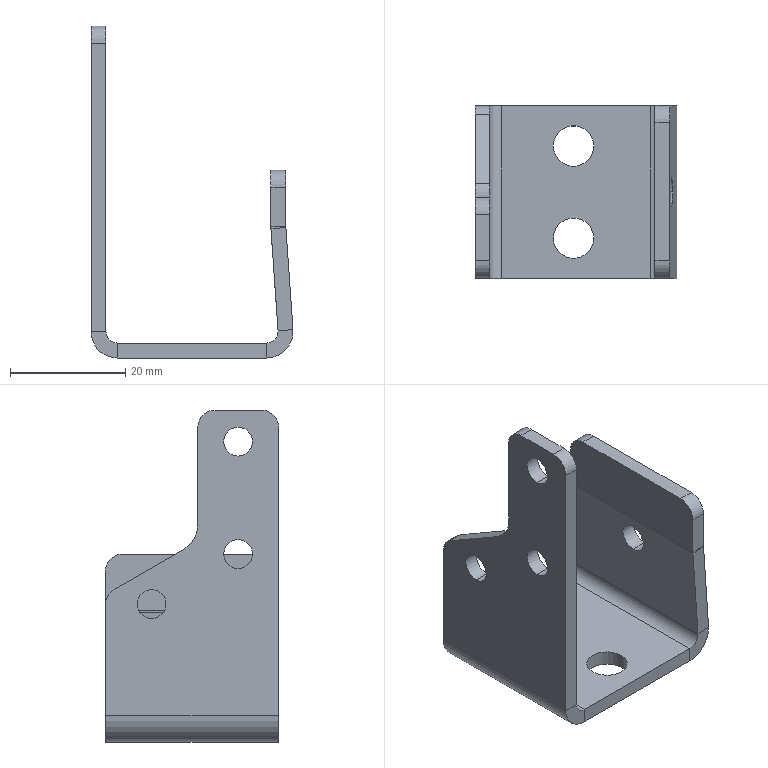Part | STEP file | SOPORTE RESORTE 1 | 1 solid | 50 faces | box 35.055 x 30 x 57.6 mm | volume 7586 mm3 | plane 26 | cylinder 24 | commonest cylinder face diameters 5 x8 6 x5 7 x4 4 x3 9.2 x3 10 x1
STEP:
#1=CARTESIAN_POINT('',(14.241,15.,3.502));
#2=VERTEX_POINT('',#1);
#3=CARTESIAN_POINT('',(14.59,15.,-1.486));
#4=VERTEX_POINT('',#3);
#5=CARTESIAN_POINT('',(14.416,15.,1.008));
#6=DIRECTION('',(0.9976,0.,0.06976));
#7=DIRECTION('',(0.06976,0.,-0.9976));
#8=AXIS2_PLACEMENT_3D('',#5,#6,#7);
#9=CIRCLE('',#8,2.5);
#10=EDGE_CURVE('',#2,#4,#9,.T.);
#11=ORIENTED_EDGE('',*,*,#10,.F.);
#12=CARTESIAN_POINT('',(16.835,15.,3.683));
#13=VERTEX_POINT('',#12);
#14=CARTESIAN_POINT('',(16.835,15.,3.683));
#15=DIRECTION('',(0.9976,0.,0.06976));
#16=VECTOR('',#15,1000.);
#17=LINE('',#14,#16);
#18=EDGE_CURVE('',#2,#13,#17,.T.);
#19=ORIENTED_EDGE('',*,*,#18,.T.);
#20=CARTESIAN_POINT('',(17.184,15.,-1.305));
#21=VERTEX_POINT('',#20);
#22=CARTESIAN_POINT('',(17.009,15.,1.189));
#23=DIRECTION('',(0.9976,0.,0.06976));
#24=DIRECTION('',(0.06976,0.,-0.9976));
#25=AXIS2_PLACEMENT_3D('',#22,#23,#24);
#26=CIRCLE('',#25,2.5);
#27=EDGE_CURVE('',#13,#21,#26,.T.);
#28=ORIENTED_EDGE('',*,*,#27,.T.);
#29=CARTESIAN_POINT('',(17.184,15.,-1.305));
#30=DIRECTION('',(0.9976,0.,0.06976));
#31=VECTOR('',#30,1000.);
#32=LINE('',#29,#31);
#33=EDGE_CURVE('',#4,#21,#32,.T.);
#34=ORIENTED_EDGE('',*,*,#33,.F.);
#35=EDGE_LOOP('',(#11,#19,#28,#34));
#36=FACE_OUTER_BOUND('',#35,.T.);
#37=CARTESIAN_POINT('',(17.009,15.,1.189));
#38=DIRECTION('',(0.9976,0.,0.06976));
#39=DIRECTION('',(0.06976,0.,-0.9976));
#40=AXIS2_PLACEMENT_3D('',#37,#38,#39);
#41=CYLINDRICAL_SURFACE('',#40,2.5);
#42=ADVANCED_FACE('',(#36),#41,.F.);
#43=CARTESIAN_POINT('',(3.5,23.,-14.5));
#44=VERTEX_POINT('',#43);
#45=CARTESIAN_POINT('',(-3.5,23.,-14.5));
#46=VERTEX_POINT('',#45);
#47=CARTESIAN_POINT('',(0.,23.,-14.5));
#48=DIRECTION('',(0.,0.,-1.));
#49=DIRECTION('',(-1.,0.,0.));
#50=AXIS2_PLACEMENT_3D('',#47,#48,#49);
#51=CIRCLE('',#50,3.5);
#52=EDGE_CURVE('',#44,#46,#51,.T.);
#53=ORIENTED_EDGE('',*,*,#52,.F.);
#54=CARTESIAN_POINT('',(3.5,23.,-17.1));
#55=VERTEX_POINT('',#54);
#56=CARTESIAN_POINT('',(3.5,23.,-17.1));
#57=DIRECTION('',(0.,0.,-1.));
#58=VECTOR('',#57,1000.);
#59=LINE('',#56,#58);
#60=EDGE_CURVE('',#44,#55,#59,.T.);
#61=ORIENTED_EDGE('',*,*,#60,.T.);
#62=CARTESIAN_POINT('',(-3.5,23.,-17.1));
#63=VERTEX_POINT('',#62);
#64=CARTESIAN_POINT('',(0.,23.,-17.1));
#65=DIRECTION('',(0.,0.,-1.));
#66=DIRECTION('',(-1.,0.,0.));
#67=AXIS2_PLACEMENT_3D('',#64,#65,#66);
#68=CIRCLE('',#67,3.5);
#69=EDGE_CURVE('',#55,#63,#68,.T.);
#70=ORIENTED_EDGE('',*,*,#69,.T.);
#71=CARTESIAN_POINT('',(-3.5,23.,-17.1));
#72=DIRECTION('',(0.,0.,-1.));
#73=VECTOR('',#72,1000.);
#74=LINE('',#71,#73);
#75=EDGE_CURVE('',#46,#63,#74,.T.);
#76=ORIENTED_EDGE('',*,*,#75,.F.);
#77=EDGE_LOOP('',(#53,#61,#70,#76));
#78=FACE_OUTER_BOUND('',#77,.T.);
#79=CARTESIAN_POINT('',(0.,23.,-17.1));
#80=DIRECTION('',(0.,0.,-1.));
#81=DIRECTION('',(-1.,0.,0.));
#82=AXIS2_PLACEMENT_3D('',#79,#80,#81);
#83=CYLINDRICAL_SURFACE('',#82,3.5);
#84=ADVANCED_FACE('',(#78),#83,.F.);
#85=CARTESIAN_POINT('',(3.5,7.,-14.5));
#86=VERTEX_POINT('',#85);
#87=CARTESIAN_POINT('',(-3.5,7.,-14.5));
#88=VERTEX_POINT('',#87);
#89=CARTESIAN_POINT('',(0.,7.,-14.5));
#90=DIRECTION('',(0.,0.,-1.));
#91=DIRECTION('',(-1.,0.,0.));
#92=AXIS2_PLACEMENT_3D('',#89,#90,#91);
#93=CIRCLE('',#92,3.5);
#94=EDGE_CURVE('',#86,#88,#93,.T.);
#95=ORIENTED_EDGE('',*,*,#94,.F.);
#96=CARTESIAN_POINT('',(3.5,7.,-17.1));
#97=VERTEX_POINT('',#96);
#98=CARTESIAN_POINT('',(3.5,7.,-17.1));
#99=DIRECTION('',(0.,0.,-1.));
#100=VECTOR('',#99,1000.);
#101=LINE('',#98,#100);
#102=EDGE_CURVE('',#86,#97,#101,.T.);
#103=ORIENTED_EDGE('',*,*,#102,.T.);
#104=CARTESIAN_POINT('',(-3.5,7.,-17.1));
#105=VERTEX_POINT('',#104);
#106=CARTESIAN_POINT('',(0.,7.,-17.1));
#107=DIRECTION('',(0.,0.,-1.));
#108=DIRECTION('',(-1.,0.,0.));
#109=AXIS2_PLACEMENT_3D('',#106,#107,#108);
#110=CIRCLE('',#109,3.5);
#111=EDGE_CURVE('',#97,#105,#110,.T.);
#112=ORIENTED_EDGE('',*,*,#111,.T.);
#113=CARTESIAN_POINT('',(-3.5,7.,-17.1));
#114=DIRECTION('',(0.,0.,-1.));
#115=VECTOR('',#114,1000.);
#116=LINE('',#113,#115);
#117=EDGE_CURVE('',#88,#105,#116,.T.);
#118=ORIENTED_EDGE('',*,*,#117,.F.);
#119=EDGE_LOOP('',(#95,#103,#112,#118));
#120=FACE_OUTER_BOUND('',#119,.T.);
#121=CARTESIAN_POINT('',(0.,7.,-17.1));
#122=DIRECTION('',(0.,0.,-1.));
#123=DIRECTION('',(-1.,0.,0.));
#124=AXIS2_PLACEMENT_3D('',#121,#122,#123);
#125=CYLINDRICAL_SURFACE('',#124,3.5);
#126=ADVANCED_FACE('',(#120),#125,.F.);
#127=CARTESIAN_POINT('',(-17.1,7.,37.5));
#128=VERTEX_POINT('',#127);
#129=CARTESIAN_POINT('',(-17.1,7.,32.5));
#130=VERTEX_POINT('',#129);
#131=CARTESIAN_POINT('',(-17.1,7.,35.));
#132=DIRECTION('',(1.,0.,0.));
#133=DIRECTION('',(0.,0.,-1.));
#134=AXIS2_PLACEMENT_3D('',#131,#132,#133);
#135=CIRCLE('',#134,2.5);
#136=EDGE_CURVE('',#128,#130,#135,.T.);
#137=ORIENTED_EDGE('',*,*,#136,.F.);
#138=CARTESIAN_POINT('',(-14.5,7.,37.5));
#139=VERTEX_POINT('',#138);
#140=CARTESIAN_POINT('',(-14.5,7.,37.5));
#141=DIRECTION('',(1.,0.,0.));
#142=VECTOR('',#141,1000.);
#143=LINE('',#140,#142);
#144=EDGE_CURVE('',#128,#139,#143,.T.);
#145=ORIENTED_EDGE('',*,*,#144,.T.);
#146=CARTESIAN_POINT('',(-14.5,7.,32.5));
#147=VERTEX_POINT('',#146);
#148=CARTESIAN_POINT('',(-14.5,7.,35.));
#149=DIRECTION('',(1.,0.,0.));
#150=DIRECTION('',(0.,0.,-1.));
#151=AXIS2_PLACEMENT_3D('',#148,#149,#150);
#152=CIRCLE('',#151,2.5);
#153=EDGE_CURVE('',#139,#147,#152,.T.);
#154=ORIENTED_EDGE('',*,*,#153,.T.);
#155=CARTESIAN_POINT('',(-14.5,7.,32.5));
#156=DIRECTION('',(1.,0.,0.));
#157=VECTOR('',#156,1000.);
#158=LINE('',#155,#157);
#159=EDGE_CURVE('',#130,#147,#158,.T.);
#160=ORIENTED_EDGE('',*,*,#159,.F.);
#161=EDGE_LOOP('',(#137,#145,#154,#160));
#162=FACE_OUTER_BOUND('',#161,.T.);
#163=CARTESIAN_POINT('',(-14.5,7.,35.));
#164=DIRECTION('',(1.,0.,0.));
#165=DIRECTION('',(0.,0.,-1.));
#166=AXIS2_PLACEMENT_3D('',#163,#164,#165);
#167=CYLINDRICAL_SURFACE('',#166,2.5);
#168=ADVANCED_FACE('',(#162),#167,.F.);
#169=CARTESIAN_POINT('',(-17.1,7.,18.));
#170=VERTEX_POINT('',#169);
#171=CARTESIAN_POINT('',(-17.1,7.,13.));
#172=VERTEX_POINT('',#171);
#173=CARTESIAN_POINT('',(-17.1,7.,15.5));
#174=DIRECTION('',(1.,0.,0.));
#175=DIRECTION('',(0.,0.,-1.));
#176=AXIS2_PLACEMENT_3D('',#173,#174,#175);
#177=CIRCLE('',#176,2.5);
#178=EDGE_CURVE('',#170,#172,#177,.T.);
#179=ORIENTED_EDGE('',*,*,#178,.F.);
#180=CARTESIAN_POINT('',(-14.5,7.,18.));
#181=VERTEX_POINT('',#180);
#182=CARTESIAN_POINT('',(-14.5,7.,18.));
#183=DIRECTION('',(1.,0.,0.));
#184=VECTOR('',#183,1000.);
#185=LINE('',#182,#184);
#186=EDGE_CURVE('',#170,#181,#185,.T.);
#187=ORIENTED_EDGE('',*,*,#186,.T.);
#188=CARTESIAN_POINT('',(-14.5,7.,13.));
#189=VERTEX_POINT('',#188);
#190=CARTESIAN_POINT('',(-14.5,7.,15.5));
#191=DIRECTION('',(1.,0.,0.));
#192=DIRECTION('',(0.,0.,-1.));
#193=AXIS2_PLACEMENT_3D('',#190,#191,#192);
#194=CIRCLE('',#193,2.5);
#195=EDGE_CURVE('',#181,#189,#194,.T.);
#196=ORIENTED_EDGE('',*,*,#195,.T.);
#197=CARTESIAN_POINT('',(-14.5,7.,13.));
#198=DIRECTION('',(1.,0.,0.));
#199=VECTOR('',#198,1000.);
#200=LINE('',#197,#199);
#201=EDGE_CURVE('',#172,#189,#200,.T.);
#202=ORIENTED_EDGE('',*,*,#201,.F.);
#203=EDGE_LOOP('',(#179,#187,#196,#202));
#204=FACE_OUTER_BOUND('',#203,.T.);
#205=CARTESIAN_POINT('',(-14.5,7.,15.5));
#206=DIRECTION('',(1.,0.,0.));
#207=DIRECTION('',(0.,0.,-1.));
#208=AXIS2_PLACEMENT_3D('',#205,#206,#207);
#209=CYLINDRICAL_SURFACE('',#208,2.5);
#210=ADVANCED_FACE('',(#204),#209,.F.);
#211=CARTESIAN_POINT('',(-17.1,22.,9.34));
#212=VERTEX_POINT('',#211);
#213=CARTESIAN_POINT('',(-17.1,22.,4.34));
#214=VERTEX_POINT('',#213);
#215=CARTESIAN_POINT('',(-17.1,22.,6.84));
#216=DIRECTION('',(1.,0.,0.));
#217=DIRECTION('',(0.,0.,-1.));
#218=AXIS2_PLACEMENT_3D('',#215,#216,#217);
#219=CIRCLE('',#218,2.5);
#220=EDGE_CURVE('',#212,#214,#219,.T.);
#221=ORIENTED_EDGE('',*,*,#220,.F.);
#222=CARTESIAN_POINT('',(-14.5,22.,9.34));
#223=VERTEX_POINT('',#222);
#224=CARTESIAN_POINT('',(-14.5,22.,9.34));
#225=DIRECTION('',(1.,0.,0.));
#226=VECTOR('',#225,1000.);
#227=LINE('',#224,#226);
#228=EDGE_CURVE('',#212,#223,#227,.T.);
#229=ORIENTED_EDGE('',*,*,#228,.T.);
#230=CARTESIAN_POINT('',(-14.5,22.,4.34));
#231=VERTEX_POINT('',#230);
#232=CARTESIAN_POINT('',(-14.5,22.,6.84));
#233=DIRECTION('',(1.,0.,0.));
#234=DIRECTION('',(0.,0.,-1.));
#235=AXIS2_PLACEMENT_3D('',#232,#233,#234);
#236=CIRCLE('',#235,2.5);
#237=EDGE_CURVE('',#223,#231,#236,.T.);
#238=ORIENTED_EDGE('',*,*,#237,.T.);
#239=CARTESIAN_POINT('',(-14.5,22.,4.34));
#240=DIRECTION('',(1.,0.,0.));
#241=VECTOR('',#240,1000.);
#242=LINE('',#239,#241);
#243=EDGE_CURVE('',#214,#231,#242,.T.);
#244=ORIENTED_EDGE('',*,*,#243,.F.);
#245=EDGE_LOOP('',(#221,#229,#238,#244));
#246=FACE_OUTER_BOUND('',#245,.T.);
#247=CARTESIAN_POINT('',(-14.5,22.,6.84));
#248=DIRECTION('',(1.,0.,0.));
#249=DIRECTION('',(0.,0.,-1.));
#250=AXIS2_PLACEMENT_3D('',#247,#248,#249);
#251=CYLINDRICAL_SURFACE('',#250,2.5);
#252=ADVANCED_FACE('',(#246),#251,.F.);
#253=CARTESIAN_POINT('',(-17.1,0.,37.5));
#254=VERTEX_POINT('',#253);
#255=CARTESIAN_POINT('',(-17.1,0.,-12.5));
#256=VERTEX_POINT('',#255);
#257=CARTESIAN_POINT('',(-17.1,0.,40.5));
#258=DIRECTION('',(0.,0.,-1.));
#259=VECTOR('',#258,1000.);
#260=LINE('',#257,#259);
#261=EDGE_CURVE('',#254,#256,#260,.T.);
#262=ORIENTED_EDGE('',*,*,#261,.F.);
#263=CARTESIAN_POINT('',(-17.1,3.,40.5));
#264=VERTEX_POINT('',#263);
#265=CARTESIAN_POINT('',(-17.1,3.,37.5));
#266=DIRECTION('',(-1.,0.,0.));
#267=DIRECTION('',(0.,0.,1.));
#268=AXIS2_PLACEMENT_3D('',#265,#266,#267);
#269=CIRCLE('',#268,3.);
#270=EDGE_CURVE('',#254,#264,#269,.T.);
#271=ORIENTED_EDGE('',*,*,#270,.T.);
#272=CARTESIAN_POINT('',(-17.1,11.,40.5));
#273=VERTEX_POINT('',#272);
#274=CARTESIAN_POINT('',(-17.1,30.,40.5));
#275=DIRECTION('',(0.,-1.,0.));
#276=VECTOR('',#275,1000.);
#277=LINE('',#274,#276);
#278=EDGE_CURVE('',#273,#264,#277,.T.);
#279=ORIENTED_EDGE('',*,*,#278,.F.);
#280=CARTESIAN_POINT('',(-17.1,14.,37.5));
#281=VERTEX_POINT('',#280);
#282=CARTESIAN_POINT('',(-17.1,11.,37.5));
#283=DIRECTION('',(-1.,0.,0.));
#284=DIRECTION('',(0.,0.,1.));
#285=AXIS2_PLACEMENT_3D('',#282,#283,#284);
#286=CIRCLE('',#285,3.);
#287=EDGE_CURVE('',#273,#281,#286,.T.);
#288=ORIENTED_EDGE('',*,*,#287,.T.);
#289=CARTESIAN_POINT('',(-17.1,14.,20.624));
#290=VERTEX_POINT('',#289);
#291=CARTESIAN_POINT('',(-17.1,14.,40.5));
#292=DIRECTION('',(0.,0.,1.));
#293=VECTOR('',#292,1000.);
#294=LINE('',#291,#293);
#295=EDGE_CURVE('',#290,#281,#294,.T.);
#296=ORIENTED_EDGE('',*,*,#295,.F.);
#297=CARTESIAN_POINT('',(-17.1,16.5,16.294));
#298=VERTEX_POINT('',#297);
#299=CARTESIAN_POINT('',(-17.1,19.,20.624));
#300=DIRECTION('',(1.,0.,0.));
#301=DIRECTION('',(0.,0.,1.));
#302=AXIS2_PLACEMENT_3D('',#299,#300,#301);
#303=CIRCLE('',#302,5.);
#304=EDGE_CURVE('',#290,#298,#303,.T.);
#305=ORIENTED_EDGE('',*,*,#304,.T.);
#306=CARTESIAN_POINT('',(-17.1,28.5,9.366));
#307=VERTEX_POINT('',#306);
#308=CARTESIAN_POINT('',(-17.1,16.144,16.5));
#309=DIRECTION('',(0.,-0.866,0.5));
#310=VECTOR('',#309,1000.);
#311=LINE('',#308,#310);
#312=EDGE_CURVE('',#307,#298,#311,.T.);
#313=ORIENTED_EDGE('',*,*,#312,.F.);
#314=CARTESIAN_POINT('',(-17.1,30.,6.768));
#315=VERTEX_POINT('',#314);
#316=CARTESIAN_POINT('',(-17.1,27.,6.768));
#317=DIRECTION('',(-1.,0.,0.));
#318=DIRECTION('',(0.,0.,1.));
#319=AXIS2_PLACEMENT_3D('',#316,#317,#318);
#320=CIRCLE('',#319,3.);
#321=EDGE_CURVE('',#307,#315,#320,.T.);
#322=ORIENTED_EDGE('',*,*,#321,.T.);
#323=CARTESIAN_POINT('',(-17.1,30.,-12.5));
#324=VERTEX_POINT('',#323);
#325=CARTESIAN_POINT('',(-17.1,30.,40.5));
#326=DIRECTION('',(0.,0.,-1.));
#327=VECTOR('',#326,1000.);
#328=LINE('',#325,#327);
#329=EDGE_CURVE('',#315,#324,#328,.T.);
#330=ORIENTED_EDGE('',*,*,#329,.T.);
#331=CARTESIAN_POINT('',(-17.1,30.,-12.5));
#332=DIRECTION('',(0.,-1.,0.));
#333=VECTOR('',#332,1000.);
#334=LINE('',#331,#333);
#335=EDGE_CURVE('',#324,#256,#334,.T.);
#336=ORIENTED_EDGE('',*,*,#335,.T.);
#337=EDGE_LOOP('',(#262,#271,#279,#288,#296,#305,#313,#322,#330,#336));
#338=FACE_OUTER_BOUND('',#337,.T.);
#339=CARTESIAN_POINT('',(-17.1,22.,6.84));
#340=DIRECTION('',(1.,0.,0.));
#341=DIRECTION('',(0.,0.,-1.));
#342=AXIS2_PLACEMENT_3D('',#339,#340,#341);
#343=CIRCLE('',#342,2.5);
#344=EDGE_CURVE('',#214,#212,#343,.T.);
#345=ORIENTED_EDGE('',*,*,#344,.T.);
#346=ORIENTED_EDGE('',*,*,#220,.T.);
#347=EDGE_LOOP('',(#345,#346));
#348=FACE_BOUND('',#347,.T.);
#349=CARTESIAN_POINT('',(-17.1,7.,15.5));
#350=DIRECTION('',(1.,0.,0.));
#351=DIRECTION('',(0.,0.,-1.));
#352=AXIS2_PLACEMENT_3D('',#349,#350,#351);
#353=CIRCLE('',#352,2.5);
#354=EDGE_CURVE('',#172,#170,#353,.T.);
#355=ORIENTED_EDGE('',*,*,#354,.T.);
#356=ORIENTED_EDGE('',*,*,#178,.T.);
#357=EDGE_LOOP('',(#355,#356));
#358=FACE_BOUND('',#357,.T.);
#359=CARTESIAN_POINT('',(-17.1,7.,35.));
#360=DIRECTION('',(1.,0.,0.));
#361=DIRECTION('',(0.,0.,-1.));
#362=AXIS2_PLACEMENT_3D('',#359,#360,#361);
#363=CIRCLE('',#362,2.5);
#364=EDGE_CURVE('',#130,#128,#363,.T.);
#365=ORIENTED_EDGE('',*,*,#364,.T.);
#366=ORIENTED_EDGE('',*,*,#136,.T.);
#367=EDGE_LOOP('',(#365,#366));
#368=FACE_BOUND('',#367,.T.);
#369=CARTESIAN_POINT('',(-17.1,30.,40.5));
#370=DIRECTION('',(-1.,0.,0.));
#371=DIRECTION('',(0.,0.,1.));
#372=AXIS2_PLACEMENT_3D('',#369,#370,#371);
#373=PLANE('',#372);
#374=ADVANCED_FACE('',(#338,#348,#358,#368),#373,.T.);
#375=ORIENTED_EDGE('',*,*,#329,.F.);
#376=CARTESIAN_POINT('',(-14.5,30.,6.768));
#377=VERTEX_POINT('',#376);
#378=CARTESIAN_POINT('',(-12.5,30.,6.768));
#379=DIRECTION('',(1.,0.,0.));
#380=VECTOR('',#379,1000.);
#381=LINE('',#378,#380);
#382=EDGE_CURVE('',#315,#377,#381,.T.);
#383=ORIENTED_EDGE('',*,*,#382,.T.);
#384=CARTESIAN_POINT('',(-14.5,30.,-12.5));
#385=VERTEX_POINT('',#384);
#386=CARTESIAN_POINT('',(-14.5,30.,40.5));
#387=DIRECTION('',(0.,0.,-1.));
#388=VECTOR('',#387,1000.);
#389=LINE('',#386,#388);
#390=EDGE_CURVE('',#377,#385,#389,.T.);
#391=ORIENTED_EDGE('',*,*,#390,.T.);
#392=CARTESIAN_POINT('',(-14.5,30.,-12.5));
#393=DIRECTION('',(-1.,0.,0.));
#394=VECTOR('',#393,1000.);
#395=LINE('',#392,#394);
#396=EDGE_CURVE('',#385,#324,#395,.T.);
#397=ORIENTED_EDGE('',*,*,#396,.T.);
#398=EDGE_LOOP('',(#375,#383,#391,#397));
#399=FACE_OUTER_BOUND('',#398,.T.);
#400=CARTESIAN_POINT('',(-12.5,30.,-17.1));
#401=DIRECTION('',(0.,1.,0.));
#402=DIRECTION('',(0.,0.,1.));
#403=AXIS2_PLACEMENT_3D('',#400,#401,#402);
#404=PLANE('',#403);
#405=ADVANCED_FACE('',(#399),#404,.T.);
#406=ORIENTED_EDGE('',*,*,#278,.T.);
#407=CARTESIAN_POINT('',(-14.5,3.,40.5));
#408=VERTEX_POINT('',#407);
#409=CARTESIAN_POINT('',(-14.5,3.,40.5));
#410=DIRECTION('',(1.,0.,0.));
#411=VECTOR('',#410,1000.);
#412=LINE('',#409,#411);
#413=EDGE_CURVE('',#264,#408,#412,.T.);
#414=ORIENTED_EDGE('',*,*,#413,.T.);
#415=CARTESIAN_POINT('',(-14.5,11.,40.5));
#416=VERTEX_POINT('',#415);
#417=CARTESIAN_POINT('',(-14.5,30.,40.5));
#418=DIRECTION('',(0.,-1.,0.));
#419=VECTOR('',#418,1000.);
#420=LINE('',#417,#419);
#421=EDGE_CURVE('',#416,#408,#420,.T.);
#422=ORIENTED_EDGE('',*,*,#421,.F.);
#423=CARTESIAN_POINT('',(-14.5,11.,40.5));
#424=DIRECTION('',(-1.,0.,0.));
#425=VECTOR('',#424,1000.);
#426=LINE('',#423,#425);
#427=EDGE_CURVE('',#416,#273,#426,.T.);
#428=ORIENTED_EDGE('',*,*,#427,.T.);
#429=EDGE_LOOP('',(#406,#414,#422,#428));
#430=FACE_OUTER_BOUND('',#429,.T.);
#431=CARTESIAN_POINT('',(-14.5,30.,40.5));
#432=DIRECTION('',(0.,0.,1.));
#433=DIRECTION('',(1.,0.,0.));
#434=AXIS2_PLACEMENT_3D('',#431,#432,#433);
#435=PLANE('',#434);
#436=ADVANCED_FACE('',(#430),#435,.T.);
#437=CARTESIAN_POINT('',(-14.5,7.,35.));
#438=DIRECTION('',(1.,0.,0.));
#439=DIRECTION('',(0.,0.,-1.));
#440=AXIS2_PLACEMENT_3D('',#437,#438,#439);
#441=CIRCLE('',#440,2.5);
#442=EDGE_CURVE('',#147,#139,#441,.T.);
#443=ORIENTED_EDGE('',*,*,#442,.F.);
#444=ORIENTED_EDGE('',*,*,#153,.F.);
#445=EDGE_LOOP('',(#443,#444));
#446=FACE_BOUND('',#445,.T.);
#447=CARTESIAN_POINT('',(-14.5,7.,15.5));
#448=DIRECTION('',(1.,0.,0.));
#449=DIRECTION('',(0.,0.,-1.));
#450=AXIS2_PLACEMENT_3D('',#447,#448,#449);
#451=CIRCLE('',#450,2.5);
#452=EDGE_CURVE('',#189,#181,#451,.T.);
#453=ORIENTED_EDGE('',*,*,#452,.F.);
#454=ORIENTED_EDGE('',*,*,#195,.F.);
#455=EDGE_LOOP('',(#453,#454));
#456=FACE_BOUND('',#455,.T.);
#457=CARTESIAN_POINT('',(-14.5,22.,6.84));
#458=DIRECTION('',(1.,0.,0.));
#459=DIRECTION('',(0.,0.,-1.));
#460=AXIS2_PLACEMENT_3D('',#457,#458,#459);
#461=CIRCLE('',#460,2.5);
#462=EDGE_CURVE('',#231,#223,#461,.T.);
#463=ORIENTED_EDGE('',*,*,#462,.F.);
#464=ORIENTED_EDGE('',*,*,#237,.F.);
#465=EDGE_LOOP('',(#463,#464));
#466=FACE_BOUND('',#465,.T.);
#467=ORIENTED_EDGE('',*,*,#421,.T.);
#468=CARTESIAN_POINT('',(-14.5,0.,37.5));
#469=VERTEX_POINT('',#468);
#470=CARTESIAN_POINT('',(-14.5,3.,37.5));
#471=DIRECTION('',(1.,0.,0.));
#472=DIRECTION('',(0.,0.,1.));
#473=AXIS2_PLACEMENT_3D('',#470,#471,#472);
#474=CIRCLE('',#473,3.);
#475=EDGE_CURVE('',#408,#469,#474,.T.);
#476=ORIENTED_EDGE('',*,*,#475,.T.);
#477=CARTESIAN_POINT('',(-14.5,0.,-12.5));
#478=VERTEX_POINT('',#477);
#479=CARTESIAN_POINT('',(-14.5,0.,40.5));
#480=DIRECTION('',(0.,0.,-1.));
#481=VECTOR('',#480,1000.);
#482=LINE('',#479,#481);
#483=EDGE_CURVE('',#469,#478,#482,.T.);
#484=ORIENTED_EDGE('',*,*,#483,.T.);
#485=CARTESIAN_POINT('',(-14.5,30.,-12.5));
#486=DIRECTION('',(0.,-1.,0.));
#487=VECTOR('',#486,1000.);
#488=LINE('',#485,#487);
#489=EDGE_CURVE('',#385,#478,#488,.T.);
#490=ORIENTED_EDGE('',*,*,#489,.F.);
#491=ORIENTED_EDGE('',*,*,#390,.F.);
#492=CARTESIAN_POINT('',(-14.5,28.5,9.366));
#493=VERTEX_POINT('',#492);
#494=CARTESIAN_POINT('',(-14.5,27.,6.768));
#495=DIRECTION('',(1.,0.,0.));
#496=DIRECTION('',(0.,0.,1.));
#497=AXIS2_PLACEMENT_3D('',#494,#495,#496);
#498=CIRCLE('',#497,3.);
#499=EDGE_CURVE('',#377,#493,#498,.T.);
#500=ORIENTED_EDGE('',*,*,#499,.T.);
#501=CARTESIAN_POINT('',(-14.5,16.5,16.294));
#502=VERTEX_POINT('',#501);
#503=CARTESIAN_POINT('',(-14.5,16.144,16.5));
#504=DIRECTION('',(0.,-0.866,0.5));
#505=VECTOR('',#504,1000.);
#506=LINE('',#503,#505);
#507=EDGE_CURVE('',#493,#502,#506,.T.);
#508=ORIENTED_EDGE('',*,*,#507,.T.);
#509=CARTESIAN_POINT('',(-14.5,14.,20.624));
#510=VERTEX_POINT('',#509);
#511=CARTESIAN_POINT('',(-14.5,19.,20.624));
#512=DIRECTION('',(-1.,0.,0.));
#513=DIRECTION('',(0.,0.,1.));
#514=AXIS2_PLACEMENT_3D('',#511,#512,#513);
#515=CIRCLE('',#514,5.);
#516=EDGE_CURVE('',#502,#510,#515,.T.);
#517=ORIENTED_EDGE('',*,*,#516,.T.);
#518=CARTESIAN_POINT('',(-14.5,14.,37.5));
#519=VERTEX_POINT('',#518);
#520=CARTESIAN_POINT('',(-14.5,14.,40.5));
#521=DIRECTION('',(0.,0.,1.));
#522=VECTOR('',#521,1000.);
#523=LINE('',#520,#522);
#524=EDGE_CURVE('',#510,#519,#523,.T.);
#525=ORIENTED_EDGE('',*,*,#524,.T.);
#526=CARTESIAN_POINT('',(-14.5,11.,37.5));
#527=DIRECTION('',(1.,0.,0.));
#528=DIRECTION('',(0.,0.,1.));
#529=AXIS2_PLACEMENT_3D('',#526,#527,#528);
#530=CIRCLE('',#529,3.);
#531=EDGE_CURVE('',#519,#416,#530,.T.);
#532=ORIENTED_EDGE('',*,*,#531,.T.);
#533=EDGE_LOOP('',(#467,#476,#484,#490,#491,#500,#508,#517,#525,#532));
#534=FACE_OUTER_BOUND('',#533,.T.);
#535=CARTESIAN_POINT('',(-14.5,30.,40.5));
#536=DIRECTION('',(-1.,0.,0.));
#537=DIRECTION('',(0.,0.,1.));
#538=AXIS2_PLACEMENT_3D('',#535,#536,#537);
#539=PLANE('',#538);
#540=ADVANCED_FACE('',(#446,#456,#466,#534),#539,.F.);
#541=ORIENTED_EDGE('',*,*,#396,.F.);
#542=CARTESIAN_POINT('',(-12.5,30.,-14.5));
#543=VERTEX_POINT('',#542);
#544=CARTESIAN_POINT('',(-12.5,30.,-12.5));
#545=DIRECTION('',(0.,-1.,0.));
#546=DIRECTION('',(0.,0.,1.));
#547=AXIS2_PLACEMENT_3D('',#544,#545,#546);
#548=CIRCLE('',#547,2.);
#549=EDGE_CURVE('',#385,#543,#548,.T.);
#550=ORIENTED_EDGE('',*,*,#549,.T.);
#551=CARTESIAN_POINT('',(-12.5,30.,-17.1));
#552=VERTEX_POINT('',#551);
#553=CARTESIAN_POINT('',(-12.5,30.,-17.1));
#554=DIRECTION('',(0.,0.,1.));
#555=VECTOR('',#554,1000.);
#556=LINE('',#553,#555);
#557=EDGE_CURVE('',#552,#543,#556,.T.);
#558=ORIENTED_EDGE('',*,*,#557,.F.);
#559=CARTESIAN_POINT('',(-12.5,30.,-12.5));
#560=DIRECTION('',(0.,-1.,0.));
#561=DIRECTION('',(1.,0.,0.));
#562=AXIS2_PLACEMENT_3D('',#559,#560,#561);
#563=CIRCLE('',#562,4.6);
#564=EDGE_CURVE('',#324,#552,#563,.T.);
#565=ORIENTED_EDGE('',*,*,#564,.F.);
#566=EDGE_LOOP('',(#541,#550,#558,#565));
#567=FACE_OUTER_BOUND('',#566,.T.);
#568=CARTESIAN_POINT('',(-14.5,30.,-12.5));
#569=DIRECTION('',(0.,1.,0.));
#570=DIRECTION('',(0.,0.,1.));
#571=AXIS2_PLACEMENT_3D('',#568,#569,#570);
#572=PLANE('',#571);
#573=ADVANCED_FACE('',(#567),#572,.T.);
#574=CARTESIAN_POINT('',(-12.5,0.,-14.5));
#575=VERTEX_POINT('',#574);
#576=CARTESIAN_POINT('',(-12.5,0.,-17.1));
#577=VERTEX_POINT('',#576);
#578=CARTESIAN_POINT('',(-12.5,0.,-14.5));
#579=DIRECTION('',(0.,0.,-1.));
#580=VECTOR('',#579,1000.);
#581=LINE('',#578,#580);
#582=EDGE_CURVE('',#575,#577,#581,.T.);
#583=ORIENTED_EDGE('',*,*,#582,.F.);
#584=CARTESIAN_POINT('',(-12.5,0.,-12.5));
#585=DIRECTION('',(0.,-1.,0.));
#586=DIRECTION('',(0.,0.,1.));
#587=AXIS2_PLACEMENT_3D('',#584,#585,#586);
#588=CIRCLE('',#587,2.);
#589=EDGE_CURVE('',#478,#575,#588,.T.);
#590=ORIENTED_EDGE('',*,*,#589,.F.);
#591=CARTESIAN_POINT('',(-17.1,0.,-12.5));
#592=DIRECTION('',(1.,0.,0.));
#593=VECTOR('',#592,1000.);
#594=LINE('',#591,#593);
#595=EDGE_CURVE('',#256,#478,#594,.T.);
#596=ORIENTED_EDGE('',*,*,#595,.F.);
#597=CARTESIAN_POINT('',(-12.5,0.,-12.5));
#598=DIRECTION('',(0.,-1.,0.));
#599=DIRECTION('',(1.,0.,0.));
#600=AXIS2_PLACEMENT_3D('',#597,#598,#599);
#601=CIRCLE('',#600,4.6);
#602=EDGE_CURVE('',#256,#577,#601,.T.);
#603=ORIENTED_EDGE('',*,*,#602,.T.);
#604=EDGE_LOOP('',(#583,#590,#596,#603));
#605=FACE_OUTER_BOUND('',#604,.T.);
#606=CARTESIAN_POINT('',(-12.5,0.,-14.5));
#607=DIRECTION('',(0.,-1.,0.));
#608=DIRECTION('',(0.,0.,-1.));
#609=AXIS2_PLACEMENT_3D('',#606,#607,#608);
#610=PLANE('',#609);
#611=ADVANCED_FACE('',(#605),#610,.T.);
#612=CARTESIAN_POINT('',(13.355,0.,-14.5));
#613=VERTEX_POINT('',#612);
#614=CARTESIAN_POINT('',(-14.5,0.,-14.5));
#615=DIRECTION('',(1.,0.,0.));
#616=VECTOR('',#615,1000.);
#617=LINE('',#614,#616);
#618=EDGE_CURVE('',#575,#613,#617,.T.);
#619=ORIENTED_EDGE('',*,*,#618,.F.);
#620=ORIENTED_EDGE('',*,*,#582,.T.);
#621=CARTESIAN_POINT('',(13.355,0.,-17.1));
#622=VERTEX_POINT('',#621);
#623=CARTESIAN_POINT('',(-14.5,0.,-17.1));
#624=DIRECTION('',(1.,0.,0.));
#625=VECTOR('',#624,1000.);
#626=LINE('',#623,#625);
#627=EDGE_CURVE('',#577,#622,#626,.T.);
#628=ORIENTED_EDGE('',*,*,#627,.T.);
#629=CARTESIAN_POINT('',(13.355,0.,-17.1));
#630=DIRECTION('',(0.,0.,1.));
#631=VECTOR('',#630,1000.);
#632=LINE('',#629,#631);
#633=EDGE_CURVE('',#622,#613,#632,.T.);
#634=ORIENTED_EDGE('',*,*,#633,.T.);
#635=EDGE_LOOP('',(#619,#620,#628,#634));
#636=FACE_OUTER_BOUND('',#635,.T.);
#637=CARTESIAN_POINT('',(-17.1,0.,-12.5));
#638=DIRECTION('',(0.,-1.,0.));
#639=DIRECTION('',(0.,0.,-1.));
#640=AXIS2_PLACEMENT_3D('',#637,#638,#639);
#641=PLANE('',#640);
#642=ADVANCED_FACE('',(#636),#641,.T.);
#643=CARTESIAN_POINT('',(13.355,30.,-14.5));
#644=VERTEX_POINT('',#643);
#645=CARTESIAN_POINT('',(13.355,30.,-17.1));
#646=VERTEX_POINT('',#645);
#647=CARTESIAN_POINT('',(13.355,30.,-14.5));
#648=DIRECTION('',(0.,0.,-1.));
#649=VECTOR('',#648,1000.);
#650=LINE('',#647,#649);
#651=EDGE_CURVE('',#644,#646,#650,.T.);
#652=ORIENTED_EDGE('',*,*,#651,.F.);
#653=CARTESIAN_POINT('',(15.35,30.,-12.36));
#654=VERTEX_POINT('',#653);
#655=CARTESIAN_POINT('',(13.355,30.,-12.5));
#656=DIRECTION('',(0.,-1.,0.));
#657=DIRECTION('',(0.,0.,1.));
#658=AXIS2_PLACEMENT_3D('',#655,#656,#657);
#659=CIRCLE('',#658,2.);
#660=EDGE_CURVE('',#644,#654,#659,.T.);
#661=ORIENTED_EDGE('',*,*,#660,.T.);
#662=CARTESIAN_POINT('',(17.944,30.,-12.179));
#663=VERTEX_POINT('',#662);
#664=CARTESIAN_POINT('',(17.944,30.,-12.179));
#665=DIRECTION('',(-0.9976,0.,-0.06976));
#666=VECTOR('',#665,1000.);
#667=LINE('',#664,#666);
#668=EDGE_CURVE('',#663,#654,#667,.T.);
#669=ORIENTED_EDGE('',*,*,#668,.F.);
#670=CARTESIAN_POINT('',(13.355,30.,-12.5));
#671=DIRECTION('',(0.,-1.,0.));
#672=DIRECTION('',(1.,0.,0.));
#673=AXIS2_PLACEMENT_3D('',#670,#671,#672);
#674=CIRCLE('',#673,4.6);
#675=EDGE_CURVE('',#646,#663,#674,.T.);
#676=ORIENTED_EDGE('',*,*,#675,.F.);
#677=EDGE_LOOP('',(#652,#661,#669,#676));
#678=FACE_OUTER_BOUND('',#677,.T.);
#679=CARTESIAN_POINT('',(13.355,30.,-14.5));
#680=DIRECTION('',(0.,1.,0.));
#681=DIRECTION('',(0.,0.,1.));
#682=AXIS2_PLACEMENT_3D('',#679,#680,#681);
#683=PLANE('',#682);
#684=ADVANCED_FACE('',(#678),#683,.T.);
#685=CARTESIAN_POINT('',(-14.5,30.,-14.5));
#686=DIRECTION('',(1.,0.,0.));
#687=VECTOR('',#686,1000.);
#688=LINE('',#685,#687);
#689=EDGE_CURVE('',#543,#644,#688,.T.);
#690=ORIENTED_EDGE('',*,*,#689,.T.);
#691=ORIENTED_EDGE('',*,*,#651,.T.);
#692=CARTESIAN_POINT('',(-14.5,30.,-17.1));
#693=DIRECTION('',(1.,0.,0.));
#694=VECTOR('',#693,1000.);
#695=LINE('',#692,#694);
#696=EDGE_CURVE('',#552,#646,#695,.T.);
#697=ORIENTED_EDGE('',*,*,#696,.F.);
#698=ORIENTED_EDGE('',*,*,#557,.T.);
#699=EDGE_LOOP('',(#690,#691,#697,#698));
#700=FACE_OUTER_BOUND('',#699,.T.);
#701=CARTESIAN_POINT('',(17.944,30.,-12.179));
#702=DIRECTION('',(0.,1.,0.));
#703=DIRECTION('',(0.,0.,1.));
#704=AXIS2_PLACEMENT_3D('',#701,#702,#703);
#705=PLANE('',#704);
#706=ADVANCED_FACE('',(#700),#705,.T.);
#707=CARTESIAN_POINT('',(15.35,0.,-12.36));
#708=VERTEX_POINT('',#707);
#709=CARTESIAN_POINT('',(17.944,0.,-12.179));
#710=VERTEX_POINT('',#709);
#711=CARTESIAN_POINT('',(15.35,0.,-12.36));
#712=DIRECTION('',(0.9976,0.,0.06976));
#713=VECTOR('',#712,1000.);
#714=LINE('',#711,#713);
#715=EDGE_CURVE('',#708,#710,#714,.T.);
#716=ORIENTED_EDGE('',*,*,#715,.F.);
#717=CARTESIAN_POINT('',(13.355,0.,-12.5));
#718=DIRECTION('',(0.,-1.,0.));
#719=DIRECTION('',(0.,0.,1.));
#720=AXIS2_PLACEMENT_3D('',#717,#718,#719);
#721=CIRCLE('',#720,2.);
#722=EDGE_CURVE('',#613,#708,#721,.T.);
#723=ORIENTED_EDGE('',*,*,#722,.F.);
#724=ORIENTED_EDGE('',*,*,#633,.F.);
#725=CARTESIAN_POINT('',(13.355,0.,-12.5));
#726=DIRECTION('',(0.,-1.,0.));
#727=DIRECTION('',(1.,0.,0.));
#728=AXIS2_PLACEMENT_3D('',#725,#726,#727);
#729=CIRCLE('',#728,4.6);
#730=EDGE_CURVE('',#622,#710,#729,.T.);
#731=ORIENTED_EDGE('',*,*,#730,.T.);
#732=EDGE_LOOP('',(#716,#723,#724,#731));
#733=FACE_OUTER_BOUND('',#732,.T.);
#734=CARTESIAN_POINT('',(15.35,0.,-12.36));
#735=DIRECTION('',(0.,-1.,0.));
#736=DIRECTION('',(0.,0.,-1.));
#737=AXIS2_PLACEMENT_3D('',#734,#735,#736);
#738=PLANE('',#737);
#739=ADVANCED_FACE('',(#733),#738,.T.);
#740=CARTESIAN_POINT('',(14.113,0.,5.34));
#741=VERTEX_POINT('',#740);
#742=CARTESIAN_POINT('',(15.5,0.,-14.5));
#743=DIRECTION('',(-0.06976,0.,0.9976));
#744=VECTOR('',#743,1000.);
#745=LINE('',#742,#744);
#746=EDGE_CURVE('',#708,#741,#745,.T.);
#747=ORIENTED_EDGE('',*,*,#746,.F.);
#748=ORIENTED_EDGE('',*,*,#715,.T.);
#749=CARTESIAN_POINT('',(16.706,0.,5.521));
#750=VERTEX_POINT('',#749);
#751=CARTESIAN_POINT('',(18.094,0.,-14.319));
#752=DIRECTION('',(-0.06976,0.,0.9976));
#753=VECTOR('',#752,1000.);
#754=LINE('',#751,#753);
#755=EDGE_CURVE('',#710,#750,#754,.T.);
#756=ORIENTED_EDGE('',*,*,#755,.T.);
#757=CARTESIAN_POINT('',(16.706,0.,5.521));
#758=DIRECTION('',(-0.9976,0.,-0.06976));
#759=VECTOR('',#758,1000.);
#760=LINE('',#757,#759);
#761=EDGE_CURVE('',#750,#741,#760,.T.);
#762=ORIENTED_EDGE('',*,*,#761,.T.);
#763=EDGE_LOOP('',(#747,#748,#756,#762));
#764=FACE_OUTER_BOUND('',#763,.T.);
#765=CARTESIAN_POINT('',(13.355,0.,-17.1));
#766=DIRECTION('',(0.,-1.,0.));
#767=DIRECTION('',(0.,0.,-1.));
#768=AXIS2_PLACEMENT_3D('',#765,#766,#767);
#769=PLANE('',#768);
#770=ADVANCED_FACE('',(#764),#769,.T.);
#771=CARTESIAN_POINT('',(14.113,30.,5.34));
#772=VERTEX_POINT('',#771);
#773=CARTESIAN_POINT('',(16.706,30.,5.521));
#774=VERTEX_POINT('',#773);
#775=CARTESIAN_POINT('',(14.113,30.,5.34));
#776=DIRECTION('',(0.9976,0.,0.06976));
#777=VECTOR('',#776,1000.);
#778=LINE('',#775,#777);
#779=EDGE_CURVE('',#772,#774,#778,.T.);
#780=ORIENTED_EDGE('',*,*,#779,.F.);
#781=CARTESIAN_POINT('',(14.101,30.,5.661));
#782=VERTEX_POINT('',#781);
#783=CARTESIAN_POINT('',(18.701,30.,5.661));
#784=DIRECTION('',(0.,1.,0.));
#785=DIRECTION('',(0.,0.,-1.));
#786=AXIS2_PLACEMENT_3D('',#783,#784,#785);
#787=CIRCLE('',#786,4.6);
#788=EDGE_CURVE('',#772,#782,#787,.T.);
#789=ORIENTED_EDGE('',*,*,#788,.T.);
#790=CARTESIAN_POINT('',(16.701,30.,5.661));
#791=VERTEX_POINT('',#790);
#792=CARTESIAN_POINT('',(16.701,30.,5.661));
#793=DIRECTION('',(-1.,0.,0.));
#794=VECTOR('',#793,1000.);
#795=LINE('',#792,#794);
#796=EDGE_CURVE('',#791,#782,#795,.T.);
#797=ORIENTED_EDGE('',*,*,#796,.F.);
#798=CARTESIAN_POINT('',(18.701,30.,5.661));
#799=DIRECTION('',(0.,1.,0.));
#800=DIRECTION('',(1.,0.,0.));
#801=AXIS2_PLACEMENT_3D('',#798,#799,#800);
#802=CIRCLE('',#801,2.);
#803=EDGE_CURVE('',#774,#791,#802,.T.);
#804=ORIENTED_EDGE('',*,*,#803,.F.);
#805=EDGE_LOOP('',(#780,#789,#797,#804));
#806=FACE_OUTER_BOUND('',#805,.T.);
#807=CARTESIAN_POINT('',(14.113,30.,5.34));
#808=DIRECTION('',(0.,1.,0.));
#809=DIRECTION('',(0.,0.,1.));
#810=AXIS2_PLACEMENT_3D('',#807,#808,#809);
#811=PLANE('',#810);
#812=ADVANCED_FACE('',(#806),#811,.T.);
#813=CARTESIAN_POINT('',(15.5,30.,-14.5));
#814=DIRECTION('',(-0.06976,0.,0.9976));
#815=VECTOR('',#814,1000.);
#816=LINE('',#813,#815);
#817=EDGE_CURVE('',#654,#772,#816,.T.);
#818=ORIENTED_EDGE('',*,*,#817,.T.);
#819=ORIENTED_EDGE('',*,*,#779,.T.);
#820=CARTESIAN_POINT('',(18.094,30.,-14.319));
#821=DIRECTION('',(-0.06976,0.,0.9976));
#822=VECTOR('',#821,1000.);
#823=LINE('',#820,#822);
#824=EDGE_CURVE('',#663,#774,#823,.T.);
#825=ORIENTED_EDGE('',*,*,#824,.F.);
#826=ORIENTED_EDGE('',*,*,#668,.T.);
#827=EDGE_LOOP('',(#818,#819,#825,#826));
#828=FACE_OUTER_BOUND('',#827,.T.);
#829=CARTESIAN_POINT('',(16.701,30.,5.661));
#830=DIRECTION('',(0.,1.,0.));
#831=DIRECTION('',(0.,0.,1.));
#832=AXIS2_PLACEMENT_3D('',#829,#830,#831);
#833=PLANE('',#832);
#834=ADVANCED_FACE('',(#828),#833,.T.);
#835=CARTESIAN_POINT('',(14.101,0.,5.661));
#836=VERTEX_POINT('',#835);
#837=CARTESIAN_POINT('',(16.701,0.,5.661));
#838=VERTEX_POINT('',#837);
#839=CARTESIAN_POINT('',(14.101,0.,5.661));
#840=DIRECTION('',(1.,0.,0.));
#841=VECTOR('',#840,1000.);
#842=LINE('',#839,#841);
#843=EDGE_CURVE('',#836,#838,#842,.T.);
#844=ORIENTED_EDGE('',*,*,#843,.F.);
#845=CARTESIAN_POINT('',(18.701,0.,5.661));
#846=DIRECTION('',(0.,1.,0.));
#847=DIRECTION('',(0.,0.,-1.));
#848=AXIS2_PLACEMENT_3D('',#845,#846,#847);
#849=CIRCLE('',#848,4.6);
#850=EDGE_CURVE('',#741,#836,#849,.T.);
#851=ORIENTED_EDGE('',*,*,#850,.F.);
#852=ORIENTED_EDGE('',*,*,#761,.F.);
#853=CARTESIAN_POINT('',(18.701,0.,5.661));
#854=DIRECTION('',(0.,1.,0.));
#855=DIRECTION('',(1.,0.,0.));
#856=AXIS2_PLACEMENT_3D('',#853,#854,#855);
#857=CIRCLE('',#856,2.);
#858=EDGE_CURVE('',#750,#838,#857,.T.);
#859=ORIENTED_EDGE('',*,*,#858,.T.);
#860=EDGE_LOOP('',(#844,#851,#852,#859));
#861=FACE_OUTER_BOUND('',#860,.T.);
#862=CARTESIAN_POINT('',(14.101,0.,5.661));
#863=DIRECTION('',(0.,-1.,0.));
#864=DIRECTION('',(0.,0.,-1.));
#865=AXIS2_PLACEMENT_3D('',#862,#863,#864);
#866=PLANE('',#865);
#867=ADVANCED_FACE('',(#861),#866,.T.);
#868=CARTESIAN_POINT('',(16.701,0.,12.5));
#869=VERTEX_POINT('',#868);
#870=CARTESIAN_POINT('',(16.701,0.,5.5));
#871=DIRECTION('',(0.,0.,1.));
#872=VECTOR('',#871,1000.);
#873=LINE('',#870,#872);
#874=EDGE_CURVE('',#838,#869,#873,.T.);
#875=ORIENTED_EDGE('',*,*,#874,.T.);
#876=CARTESIAN_POINT('',(14.101,0.,12.5));
#877=VERTEX_POINT('',#876);
#878=CARTESIAN_POINT('',(16.706,0.,12.5));
#879=DIRECTION('',(-1.,0.,0.));
#880=VECTOR('',#879,1000.);
#881=LINE('',#878,#880);
#882=EDGE_CURVE('',#869,#877,#881,.T.);
#883=ORIENTED_EDGE('',*,*,#882,.T.);
#884=CARTESIAN_POINT('',(14.101,0.,5.5));
#885=DIRECTION('',(0.,0.,1.));
#886=VECTOR('',#885,1000.);
#887=LINE('',#884,#886);
#888=EDGE_CURVE('',#836,#877,#887,.T.);
#889=ORIENTED_EDGE('',*,*,#888,.F.);
#890=ORIENTED_EDGE('',*,*,#843,.T.);
#891=EDGE_LOOP('',(#875,#883,#889,#890));
#892=FACE_OUTER_BOUND('',#891,.T.);
#893=CARTESIAN_POINT('',(16.706,0.,5.521));
#894=DIRECTION('',(0.,-1.,0.));
#895=DIRECTION('',(0.,0.,-1.));
#896=AXIS2_PLACEMENT_3D('',#893,#894,#895);
#897=PLANE('',#896);
#898=ADVANCED_FACE('',(#892),#897,.T.);
#899=ORIENTED_EDGE('',*,*,#888,.T.);
#900=CARTESIAN_POINT('',(14.101,3.,15.5));
#901=VERTEX_POINT('',#900);
#902=CARTESIAN_POINT('',(14.101,3.,12.5));
#903=DIRECTION('',(-1.,0.,0.));
#904=DIRECTION('',(0.,0.,-1.));
#905=AXIS2_PLACEMENT_3D('',#902,#903,#904);
#906=CIRCLE('',#905,3.);
#907=EDGE_CURVE('',#877,#901,#906,.T.);
#908=ORIENTED_EDGE('',*,*,#907,.T.);
#909=CARTESIAN_POINT('',(14.101,27.,15.5));
#910=VERTEX_POINT('',#909);
#911=CARTESIAN_POINT('',(14.101,30.,15.5));
#912=DIRECTION('',(0.,-1.,0.));
#913=VECTOR('',#912,1000.);
#914=LINE('',#911,#913);
#915=EDGE_CURVE('',#910,#901,#914,.T.);
#916=ORIENTED_EDGE('',*,*,#915,.F.);
#917=CARTESIAN_POINT('',(14.101,30.,12.5));
#918=VERTEX_POINT('',#917);
#919=CARTESIAN_POINT('',(14.101,27.,12.5));
#920=DIRECTION('',(-1.,0.,0.));
#921=DIRECTION('',(0.,0.,-1.));
#922=AXIS2_PLACEMENT_3D('',#919,#920,#921);
#923=CIRCLE('',#922,3.);
#924=EDGE_CURVE('',#910,#918,#923,.T.);
#925=ORIENTED_EDGE('',*,*,#924,.T.);
#926=CARTESIAN_POINT('',(14.101,30.,5.5));
#927=DIRECTION('',(0.,0.,1.));
#928=VECTOR('',#927,1000.);
#929=LINE('',#926,#928);
#930=EDGE_CURVE('',#782,#918,#929,.T.);
#931=ORIENTED_EDGE('',*,*,#930,.F.);
#932=CARTESIAN_POINT('',(14.101,30.,5.661));
#933=DIRECTION('',(0.,-1.,0.));
#934=VECTOR('',#933,1000.);
#935=LINE('',#932,#934);
#936=EDGE_CURVE('',#782,#836,#935,.T.);
#937=ORIENTED_EDGE('',*,*,#936,.T.);
#938=EDGE_LOOP('',(#899,#908,#916,#925,#931,#937));
#939=FACE_OUTER_BOUND('',#938,.T.);
#940=CARTESIAN_POINT('',(14.101,30.,5.5));
#941=DIRECTION('',(1.,0.,0.));
#942=DIRECTION('',(0.,0.,-1.));
#943=AXIS2_PLACEMENT_3D('',#940,#941,#942);
#944=PLANE('',#943);
#945=ADVANCED_FACE('',(#939),#944,.F.);
#946=ORIENTED_EDGE('',*,*,#915,.T.);
#947=CARTESIAN_POINT('',(16.701,3.,15.5));
#948=VERTEX_POINT('',#947);
#949=CARTESIAN_POINT('',(16.701,3.,15.5));
#950=DIRECTION('',(1.,0.,0.));
#951=VECTOR('',#950,1000.);
#952=LINE('',#949,#951);
#953=EDGE_CURVE('',#901,#948,#952,.T.);
#954=ORIENTED_EDGE('',*,*,#953,.T.);
#955=CARTESIAN_POINT('',(16.701,27.,15.5));
#956=VERTEX_POINT('',#955);
#957=CARTESIAN_POINT('',(16.701,30.,15.5));
#958=DIRECTION('',(0.,-1.,0.));
#959=VECTOR('',#958,1000.);
#960=LINE('',#957,#959);
#961=EDGE_CURVE('',#956,#948,#960,.T.);
#962=ORIENTED_EDGE('',*,*,#961,.F.);
#963=CARTESIAN_POINT('',(16.701,27.,15.5));
#964=DIRECTION('',(-1.,0.,0.));
#965=VECTOR('',#964,1000.);
#966=LINE('',#963,#965);
#967=EDGE_CURVE('',#956,#910,#966,.T.);
#968=ORIENTED_EDGE('',*,*,#967,.T.);
#969=EDGE_LOOP('',(#946,#954,#962,#968));
#970=FACE_OUTER_BOUND('',#969,.T.);
#971=CARTESIAN_POINT('',(16.701,30.,15.5));
#972=DIRECTION('',(0.,0.,1.));
#973=DIRECTION('',(1.,0.,0.));
#974=AXIS2_PLACEMENT_3D('',#971,#972,#973);
#975=PLANE('',#974);
#976=ADVANCED_FACE('',(#970),#975,.T.);
#977=ORIENTED_EDGE('',*,*,#961,.T.);
#978=CARTESIAN_POINT('',(16.701,3.,12.5));
#979=DIRECTION('',(1.,0.,0.));
#980=DIRECTION('',(0.,0.,-1.));
#981=AXIS2_PLACEMENT_3D('',#978,#979,#980);
#982=CIRCLE('',#981,3.);
#983=EDGE_CURVE('',#948,#869,#982,.T.);
#984=ORIENTED_EDGE('',*,*,#983,.T.);
#985=ORIENTED_EDGE('',*,*,#874,.F.);
#986=CARTESIAN_POINT('',(16.701,30.,5.661));
#987=DIRECTION('',(0.,-1.,0.));
#988=VECTOR('',#987,1000.);
#989=LINE('',#986,#988);
#990=EDGE_CURVE('',#791,#838,#989,.T.);
#991=ORIENTED_EDGE('',*,*,#990,.F.);
#992=CARTESIAN_POINT('',(16.701,30.,12.5));
#993=VERTEX_POINT('',#992);
#994=CARTESIAN_POINT('',(16.701,30.,5.5));
#995=DIRECTION('',(0.,0.,1.));
#996=VECTOR('',#995,1000.);
#997=LINE('',#994,#996);
#998=EDGE_CURVE('',#791,#993,#997,.T.);
#999=ORIENTED_EDGE('',*,*,#998,.T.);
#1000=CARTESIAN_POINT('',(16.701,27.,12.5));
#1001=DIRECTION('',(1.,0.,0.));
#1002=DIRECTION('',(0.,0.,-1.));
#1003=AXIS2_PLACEMENT_3D('',#1000,#1001,#1002);
#1004=CIRCLE('',#1003,3.);
#1005=EDGE_CURVE('',#993,#956,#1004,.T.);
#1006=ORIENTED_EDGE('',*,*,#1005,.T.);
#1007=EDGE_LOOP('',(#977,#984,#985,#991,#999,#1006));
#1008=FACE_OUTER_BOUND('',#1007,.T.);
#1009=CARTESIAN_POINT('',(16.701,30.,5.5));
#1010=DIRECTION('',(1.,0.,0.));
#1011=DIRECTION('',(0.,0.,-1.));
#1012=AXIS2_PLACEMENT_3D('',#1009,#1010,#1011);
#1013=PLANE('',#1012);
#1014=ADVANCED_FACE('',(#1008),#1013,.T.);
#1015=ORIENTED_EDGE('',*,*,#858,.F.);
#1016=CARTESIAN_POINT('',(16.706,30.,5.521));
#1017=DIRECTION('',(0.,-1.,0.));
#1018=VECTOR('',#1017,1000.);
#1019=LINE('',#1016,#1018);
#1020=EDGE_CURVE('',#774,#750,#1019,.T.);
#1021=ORIENTED_EDGE('',*,*,#1020,.F.);
#1022=ORIENTED_EDGE('',*,*,#803,.T.);
#1023=ORIENTED_EDGE('',*,*,#990,.T.);
#1024=EDGE_LOOP('',(#1015,#1021,#1022,#1023));
#1025=FACE_OUTER_BOUND('',#1024,.T.);
#1026=CARTESIAN_POINT('',(18.701,30.,5.661));
#1027=DIRECTION('',(0.,-1.,0.));
#1028=DIRECTION('',(0.,0.,-1.));
#1029=AXIS2_PLACEMENT_3D('',#1026,#1027,#1028);
#1030=CYLINDRICAL_SURFACE('',#1029,2.);
#1031=ADVANCED_FACE('',(#1025),#1030,.F.);
#1032=CARTESIAN_POINT('',(17.009,15.,1.189));
#1033=DIRECTION('',(0.9976,0.,0.06976));
#1034=DIRECTION('',(0.06976,0.,-0.9976));
#1035=AXIS2_PLACEMENT_3D('',#1032,#1033,#1034);
#1036=CIRCLE('',#1035,2.5);
#1037=EDGE_CURVE('',#21,#13,#1036,.T.);
#1038=ORIENTED_EDGE('',*,*,#1037,.F.);
#1039=ORIENTED_EDGE('',*,*,#27,.F.);
#1040=EDGE_LOOP('',(#1038,#1039));
#1041=FACE_BOUND('',#1040,.T.);
#1042=ORIENTED_EDGE('',*,*,#755,.F.);
#1043=CARTESIAN_POINT('',(17.944,30.,-12.179));
#1044=DIRECTION('',(0.,-1.,0.));
#1045=VECTOR('',#1044,1000.);
#1046=LINE('',#1043,#1045);
#1047=EDGE_CURVE('',#663,#710,#1046,.T.);
#1048=ORIENTED_EDGE('',*,*,#1047,.F.);
#1049=ORIENTED_EDGE('',*,*,#824,.T.);
#1050=ORIENTED_EDGE('',*,*,#1020,.T.);
#1051=EDGE_LOOP('',(#1042,#1048,#1049,#1050));
#1052=FACE_OUTER_BOUND('',#1051,.T.);
#1053=CARTESIAN_POINT('',(18.094,30.,-14.319));
#1054=DIRECTION('',(0.9976,0.,0.06976));
#1055=DIRECTION('',(0.06976,0.,-0.9976));
#1056=AXIS2_PLACEMENT_3D('',#1053,#1054,#1055);
#1057=PLANE('',#1056);
#1058=ADVANCED_FACE('',(#1041,#1052),#1057,.T.);
#1059=ORIENTED_EDGE('',*,*,#730,.F.);
#1060=CARTESIAN_POINT('',(13.355,30.,-17.1));
#1061=DIRECTION('',(0.,-1.,0.));
#1062=VECTOR('',#1061,1000.);
#1063=LINE('',#1060,#1062);
#1064=EDGE_CURVE('',#646,#622,#1063,.T.);
#1065=ORIENTED_EDGE('',*,*,#1064,.F.);
#1066=ORIENTED_EDGE('',*,*,#675,.T.);
#1067=ORIENTED_EDGE('',*,*,#1047,.T.);
#1068=EDGE_LOOP('',(#1059,#1065,#1066,#1067));
#1069=FACE_OUTER_BOUND('',#1068,.T.);
#1070=CARTESIAN_POINT('',(13.355,30.,-12.5));
#1071=DIRECTION('',(0.,-1.,0.));
#1072=DIRECTION('',(0.,0.,-1.));
#1073=AXIS2_PLACEMENT_3D('',#1070,#1071,#1072);
#1074=CYLINDRICAL_SURFACE('',#1073,4.6);
#1075=ADVANCED_FACE('',(#1069),#1074,.T.);
#1076=CARTESIAN_POINT('',(0.,23.,-17.1));
#1077=DIRECTION('',(0.,0.,-1.));
#1078=DIRECTION('',(-1.,0.,0.));
#1079=AXIS2_PLACEMENT_3D('',#1076,#1077,#1078);
#1080=CIRCLE('',#1079,3.5);
#1081=EDGE_CURVE('',#63,#55,#1080,.T.);
#1082=ORIENTED_EDGE('',*,*,#1081,.F.);
#1083=ORIENTED_EDGE('',*,*,#69,.F.);
#1084=EDGE_LOOP('',(#1082,#1083));
#1085=FACE_BOUND('',#1084,.T.);
#1086=CARTESIAN_POINT('',(0.,7.,-17.1));
#1087=DIRECTION('',(0.,0.,-1.));
#1088=DIRECTION('',(-1.,0.,0.));
#1089=AXIS2_PLACEMENT_3D('',#1086,#1087,#1088);
#1090=CIRCLE('',#1089,3.5);
#1091=EDGE_CURVE('',#105,#97,#1090,.T.);
#1092=ORIENTED_EDGE('',*,*,#1091,.F.);
#1093=ORIENTED_EDGE('',*,*,#111,.F.);
#1094=EDGE_LOOP('',(#1092,#1093));
#1095=FACE_BOUND('',#1094,.T.);
#1096=ORIENTED_EDGE('',*,*,#627,.F.);
#1097=CARTESIAN_POINT('',(-12.5,30.,-17.1));
#1098=DIRECTION('',(0.,-1.,0.));
#1099=VECTOR('',#1098,1000.);
#1100=LINE('',#1097,#1099);
#1101=EDGE_CURVE('',#552,#577,#1100,.T.);
#1102=ORIENTED_EDGE('',*,*,#1101,.F.);
#1103=ORIENTED_EDGE('',*,*,#696,.T.);
#1104=ORIENTED_EDGE('',*,*,#1064,.T.);
#1105=EDGE_LOOP('',(#1096,#1102,#1103,#1104));
#1106=FACE_OUTER_BOUND('',#1105,.T.);
#1107=CARTESIAN_POINT('',(-14.5,30.,-17.1));
#1108=DIRECTION('',(0.,0.,-1.));
#1109=DIRECTION('',(-1.,0.,0.));
#1110=AXIS2_PLACEMENT_3D('',#1107,#1108,#1109);
#1111=PLANE('',#1110);
#1112=ADVANCED_FACE('',(#1085,#1095,#1106),#1111,.T.);
#1113=ORIENTED_EDGE('',*,*,#602,.F.);
#1114=ORIENTED_EDGE('',*,*,#335,.F.);
#1115=ORIENTED_EDGE('',*,*,#564,.T.);
#1116=ORIENTED_EDGE('',*,*,#1101,.T.);
#1117=EDGE_LOOP('',(#1113,#1114,#1115,#1116));
#1118=FACE_OUTER_BOUND('',#1117,.T.);
#1119=CARTESIAN_POINT('',(-12.5,30.,-12.5));
#1120=DIRECTION('',(0.,-1.,0.));
#1121=DIRECTION('',(0.,0.,-1.));
#1122=AXIS2_PLACEMENT_3D('',#1119,#1120,#1121);
#1123=CYLINDRICAL_SURFACE('',#1122,4.6);
#1124=ADVANCED_FACE('',(#1118),#1123,.T.);
#1125=ORIENTED_EDGE('',*,*,#589,.T.);
#1126=CARTESIAN_POINT('',(-12.5,30.,-14.5));
#1127=DIRECTION('',(0.,-1.,0.));
#1128=VECTOR('',#1127,1000.);
#1129=LINE('',#1126,#1128);
#1130=EDGE_CURVE('',#543,#575,#1129,.T.);
#1131=ORIENTED_EDGE('',*,*,#1130,.F.);
#1132=ORIENTED_EDGE('',*,*,#549,.F.);
#1133=ORIENTED_EDGE('',*,*,#489,.T.);
#1134=EDGE_LOOP('',(#1125,#1131,#1132,#1133));
#1135=FACE_OUTER_BOUND('',#1134,.T.);
#1136=CARTESIAN_POINT('',(-12.5,30.,-12.5));
#1137=DIRECTION('',(0.,-1.,0.));
#1138=DIRECTION('',(0.,0.,-1.));
#1139=AXIS2_PLACEMENT_3D('',#1136,#1137,#1138);
#1140=CYLINDRICAL_SURFACE('',#1139,2.);
#1141=ADVANCED_FACE('',(#1135),#1140,.F.);
#1142=CARTESIAN_POINT('',(0.,23.,-14.5));
#1143=DIRECTION('',(0.,0.,-1.));
#1144=DIRECTION('',(-1.,0.,0.));
#1145=AXIS2_PLACEMENT_3D('',#1142,#1143,#1144);
#1146=CIRCLE('',#1145,3.5);
#1147=EDGE_CURVE('',#46,#44,#1146,.T.);
#1148=ORIENTED_EDGE('',*,*,#1147,.T.);
#1149=ORIENTED_EDGE('',*,*,#52,.T.);
#1150=EDGE_LOOP('',(#1148,#1149));
#1151=FACE_BOUND('',#1150,.T.);
#1152=CARTESIAN_POINT('',(0.,7.,-14.5));
#1153=DIRECTION('',(0.,0.,-1.));
#1154=DIRECTION('',(-1.,0.,0.));
#1155=AXIS2_PLACEMENT_3D('',#1152,#1153,#1154);
#1156=CIRCLE('',#1155,3.5);
#1157=EDGE_CURVE('',#88,#86,#1156,.T.);
#1158=ORIENTED_EDGE('',*,*,#1157,.T.);
#1159=ORIENTED_EDGE('',*,*,#94,.T.);
#1160=EDGE_LOOP('',(#1158,#1159));
#1161=FACE_BOUND('',#1160,.T.);
#1162=ORIENTED_EDGE('',*,*,#618,.T.);
#1163=CARTESIAN_POINT('',(13.355,30.,-14.5));
#1164=DIRECTION('',(0.,-1.,0.));
#1165=VECTOR('',#1164,1000.);
#1166=LINE('',#1163,#1165);
#1167=EDGE_CURVE('',#644,#613,#1166,.T.);
#1168=ORIENTED_EDGE('',*,*,#1167,.F.);
#1169=ORIENTED_EDGE('',*,*,#689,.F.);
#1170=ORIENTED_EDGE('',*,*,#1130,.T.);
#1171=EDGE_LOOP('',(#1162,#1168,#1169,#1170));
#1172=FACE_OUTER_BOUND('',#1171,.T.);
#1173=CARTESIAN_POINT('',(-14.5,30.,-14.5));
#1174=DIRECTION('',(0.,0.,-1.));
#1175=DIRECTION('',(-1.,0.,0.));
#1176=AXIS2_PLACEMENT_3D('',#1173,#1174,#1175);
#1177=PLANE('',#1176);
#1178=ADVANCED_FACE('',(#1151,#1161,#1172),#1177,.F.);
#1179=ORIENTED_EDGE('',*,*,#722,.T.);
#1180=CARTESIAN_POINT('',(15.35,30.,-12.36));
#1181=DIRECTION('',(0.,-1.,0.));
#1182=VECTOR('',#1181,1000.);
#1183=LINE('',#1180,#1182);
#1184=EDGE_CURVE('',#654,#708,#1183,.T.);
#1185=ORIENTED_EDGE('',*,*,#1184,.F.);
#1186=ORIENTED_EDGE('',*,*,#660,.F.);
#1187=ORIENTED_EDGE('',*,*,#1167,.T.);
#1188=EDGE_LOOP('',(#1179,#1185,#1186,#1187));
#1189=FACE_OUTER_BOUND('',#1188,.T.);
#1190=CARTESIAN_POINT('',(13.355,30.,-12.5));
#1191=DIRECTION('',(0.,-1.,0.));
#1192=DIRECTION('',(0.,0.,-1.));
#1193=AXIS2_PLACEMENT_3D('',#1190,#1191,#1192);
#1194=CYLINDRICAL_SURFACE('',#1193,2.);
#1195=ADVANCED_FACE('',(#1189),#1194,.F.);
#1196=CARTESIAN_POINT('',(14.416,15.,1.008));
#1197=DIRECTION('',(0.9976,0.,0.06976));
#1198=DIRECTION('',(0.06976,0.,-0.9976));
#1199=AXIS2_PLACEMENT_3D('',#1196,#1197,#1198);
#1200=CIRCLE('',#1199,2.5);
#1201=EDGE_CURVE('',#4,#2,#1200,.T.);
#1202=ORIENTED_EDGE('',*,*,#1201,.T.);
#1203=ORIENTED_EDGE('',*,*,#10,.T.);
#1204=EDGE_LOOP('',(#1202,#1203));
#1205=FACE_BOUND('',#1204,.T.);
#1206=ORIENTED_EDGE('',*,*,#746,.T.);
#1207=CARTESIAN_POINT('',(14.113,30.,5.34));
#1208=DIRECTION('',(0.,-1.,0.));
#1209=VECTOR('',#1208,1000.);
#1210=LINE('',#1207,#1209);
#1211=EDGE_CURVE('',#772,#741,#1210,.T.);
#1212=ORIENTED_EDGE('',*,*,#1211,.F.);
#1213=ORIENTED_EDGE('',*,*,#817,.F.);
#1214=ORIENTED_EDGE('',*,*,#1184,.T.);
#1215=EDGE_LOOP('',(#1206,#1212,#1213,#1214));
#1216=FACE_OUTER_BOUND('',#1215,.T.);
#1217=CARTESIAN_POINT('',(15.5,30.,-14.5));
#1218=DIRECTION('',(0.9976,0.,0.06976));
#1219=DIRECTION('',(0.06976,0.,-0.9976));
#1220=AXIS2_PLACEMENT_3D('',#1217,#1218,#1219);
#1221=PLANE('',#1220);
#1222=ADVANCED_FACE('',(#1205,#1216),#1221,.F.);
#1223=ORIENTED_EDGE('',*,*,#850,.T.);
#1224=ORIENTED_EDGE('',*,*,#936,.F.);
#1225=ORIENTED_EDGE('',*,*,#788,.F.);
#1226=ORIENTED_EDGE('',*,*,#1211,.T.);
#1227=EDGE_LOOP('',(#1223,#1224,#1225,#1226));
#1228=FACE_OUTER_BOUND('',#1227,.T.);
#1229=CARTESIAN_POINT('',(18.701,30.,5.661));
#1230=DIRECTION('',(0.,-1.,0.));
#1231=DIRECTION('',(0.,0.,-1.));
#1232=AXIS2_PLACEMENT_3D('',#1229,#1230,#1231);
#1233=CYLINDRICAL_SURFACE('',#1232,4.6);
#1234=ADVANCED_FACE('',(#1228),#1233,.T.);
#1235=ORIENTED_EDGE('',*,*,#930,.T.);
#1236=CARTESIAN_POINT('',(18.701,30.,12.5));
#1237=DIRECTION('',(1.,0.,0.));
#1238=VECTOR('',#1237,1000.);
#1239=LINE('',#1236,#1238);
#1240=EDGE_CURVE('',#918,#993,#1239,.T.);
#1241=ORIENTED_EDGE('',*,*,#1240,.T.);
#1242=ORIENTED_EDGE('',*,*,#998,.F.);
#1243=ORIENTED_EDGE('',*,*,#796,.T.);
#1244=EDGE_LOOP('',(#1235,#1241,#1242,#1243));
#1245=FACE_OUTER_BOUND('',#1244,.T.);
#1246=CARTESIAN_POINT('',(18.701,30.,5.661));
#1247=DIRECTION('',(0.,1.,0.));
#1248=DIRECTION('',(1.,0.,0.));
#1249=AXIS2_PLACEMENT_3D('',#1246,#1247,#1248);
#1250=PLANE('',#1249);
#1251=ADVANCED_FACE('',(#1245),#1250,.T.);
#1252=ORIENTED_EDGE('',*,*,#483,.F.);
#1253=CARTESIAN_POINT('',(-17.1,0.,37.5));
#1254=DIRECTION('',(-1.,0.,0.));
#1255=VECTOR('',#1254,1000.);
#1256=LINE('',#1253,#1255);
#1257=EDGE_CURVE('',#469,#254,#1256,.T.);
#1258=ORIENTED_EDGE('',*,*,#1257,.T.);
#1259=ORIENTED_EDGE('',*,*,#261,.T.);
#1260=ORIENTED_EDGE('',*,*,#595,.T.);
#1261=EDGE_LOOP('',(#1252,#1258,#1259,#1260));
#1262=FACE_OUTER_BOUND('',#1261,.T.);
#1263=CARTESIAN_POINT('',(18.701,0.,5.661));
#1264=DIRECTION('',(0.,1.,0.));
#1265=DIRECTION('',(1.,0.,0.));
#1266=AXIS2_PLACEMENT_3D('',#1263,#1264,#1265);
#1267=PLANE('',#1266);
#1268=ADVANCED_FACE('',(#1262),#1267,.F.);
#1269=ORIENTED_EDGE('',*,*,#983,.F.);
#1270=ORIENTED_EDGE('',*,*,#953,.F.);
#1271=ORIENTED_EDGE('',*,*,#907,.F.);
#1272=ORIENTED_EDGE('',*,*,#882,.F.);
#1273=EDGE_LOOP('',(#1269,#1270,#1271,#1272));
#1274=FACE_OUTER_BOUND('',#1273,.T.);
#1275=CARTESIAN_POINT('',(16.706,3.,12.5));
#1276=DIRECTION('',(-1.,0.,0.));
#1277=DIRECTION('',(0.,0.,1.));
#1278=AXIS2_PLACEMENT_3D('',#1275,#1276,#1277);
#1279=CYLINDRICAL_SURFACE('',#1278,3.);
#1280=ADVANCED_FACE('',(#1274),#1279,.T.);
#1281=ORIENTED_EDGE('',*,*,#1005,.F.);
#1282=ORIENTED_EDGE('',*,*,#1240,.F.);
#1283=ORIENTED_EDGE('',*,*,#924,.F.);
#1284=ORIENTED_EDGE('',*,*,#967,.F.);
#1285=EDGE_LOOP('',(#1281,#1282,#1283,#1284));
#1286=FACE_OUTER_BOUND('',#1285,.T.);
#1287=CARTESIAN_POINT('',(16.701,27.,12.5));
#1288=DIRECTION('',(-1.,0.,0.));
#1289=DIRECTION('',(0.,0.,1.));
#1290=AXIS2_PLACEMENT_3D('',#1287,#1288,#1289);
#1291=CYLINDRICAL_SURFACE('',#1290,3.);
#1292=ADVANCED_FACE('',(#1286),#1291,.T.);
#1293=ORIENTED_EDGE('',*,*,#295,.T.);
#1294=CARTESIAN_POINT('',(-14.5,14.,37.5));
#1295=DIRECTION('',(1.,0.,0.));
#1296=VECTOR('',#1295,1000.);
#1297=LINE('',#1294,#1296);
#1298=EDGE_CURVE('',#281,#519,#1297,.T.);
#1299=ORIENTED_EDGE('',*,*,#1298,.T.);
#1300=ORIENTED_EDGE('',*,*,#524,.F.);
#1301=CARTESIAN_POINT('',(-17.1,14.,20.624));
#1302=DIRECTION('',(-1.,0.,0.));
#1303=VECTOR('',#1302,1000.);
#1304=LINE('',#1301,#1303);
#1305=EDGE_CURVE('',#510,#290,#1304,.T.);
#1306=ORIENTED_EDGE('',*,*,#1305,.T.);
#1307=EDGE_LOOP('',(#1293,#1299,#1300,#1306));
#1308=FACE_OUTER_BOUND('',#1307,.T.);
#1309=CARTESIAN_POINT('',(-14.5,14.,40.5));
#1310=DIRECTION('',(0.,-1.,0.));
#1311=DIRECTION('',(0.,0.,1.));
#1312=AXIS2_PLACEMENT_3D('',#1309,#1310,#1311);
#1313=PLANE('',#1312);
#1314=ADVANCED_FACE('',(#1308),#1313,.F.);
#1315=ORIENTED_EDGE('',*,*,#507,.F.);
#1316=CARTESIAN_POINT('',(-14.5,28.5,9.366));
#1317=DIRECTION('',(-1.,0.,0.));
#1318=VECTOR('',#1317,1000.);
#1319=LINE('',#1316,#1318);
#1320=EDGE_CURVE('',#493,#307,#1319,.T.);
#1321=ORIENTED_EDGE('',*,*,#1320,.T.);
#1322=ORIENTED_EDGE('',*,*,#312,.T.);
#1323=CARTESIAN_POINT('',(-14.5,16.5,16.294));
#1324=DIRECTION('',(1.,0.,0.));
#1325=VECTOR('',#1324,1000.);
#1326=LINE('',#1323,#1325);
#1327=EDGE_CURVE('',#298,#502,#1326,.T.);
#1328=ORIENTED_EDGE('',*,*,#1327,.T.);
#1329=EDGE_LOOP('',(#1315,#1321,#1322,#1328));
#1330=FACE_OUTER_BOUND('',#1329,.T.);
#1331=CARTESIAN_POINT('',(-14.5,16.144,16.5));
#1332=DIRECTION('',(0.,-0.5,-0.866));
#1333=DIRECTION('',(0.,-0.866,0.5));
#1334=AXIS2_PLACEMENT_3D('',#1331,#1332,#1333);
#1335=PLANE('',#1334);
#1336=ADVANCED_FACE('',(#1330),#1335,.F.);
#1337=ORIENTED_EDGE('',*,*,#516,.F.);
#1338=ORIENTED_EDGE('',*,*,#1327,.F.);
#1339=ORIENTED_EDGE('',*,*,#304,.F.);
#1340=ORIENTED_EDGE('',*,*,#1305,.F.);
#1341=EDGE_LOOP('',(#1337,#1338,#1339,#1340));
#1342=FACE_OUTER_BOUND('',#1341,.T.);
#1343=CARTESIAN_POINT('',(-14.5,19.,20.624));
#1344=DIRECTION('',(1.,0.,0.));
#1345=DIRECTION('',(0.,0.,-1.));
#1346=AXIS2_PLACEMENT_3D('',#1343,#1344,#1345);
#1347=CYLINDRICAL_SURFACE('',#1346,5.);
#1348=ADVANCED_FACE('',(#1342),#1347,.F.);
#1349=ORIENTED_EDGE('',*,*,#475,.F.);
#1350=ORIENTED_EDGE('',*,*,#413,.F.);
#1351=ORIENTED_EDGE('',*,*,#270,.F.);
#1352=ORIENTED_EDGE('',*,*,#1257,.F.);
#1353=EDGE_LOOP('',(#1349,#1350,#1351,#1352));
#1354=FACE_OUTER_BOUND('',#1353,.T.);
#1355=CARTESIAN_POINT('',(18.701,3.,37.5));
#1356=DIRECTION('',(1.,0.,0.));
#1357=DIRECTION('',(0.,0.,-1.));
#1358=AXIS2_PLACEMENT_3D('',#1355,#1356,#1357);
#1359=CYLINDRICAL_SURFACE('',#1358,3.);
#1360=ADVANCED_FACE('',(#1354),#1359,.T.);
#1361=ORIENTED_EDGE('',*,*,#531,.F.);
#1362=ORIENTED_EDGE('',*,*,#1298,.F.);
#1363=ORIENTED_EDGE('',*,*,#287,.F.);
#1364=ORIENTED_EDGE('',*,*,#427,.F.);
#1365=EDGE_LOOP('',(#1361,#1362,#1363,#1364));
#1366=FACE_OUTER_BOUND('',#1365,.T.);
#1367=CARTESIAN_POINT('',(-14.5,11.,37.5));
#1368=DIRECTION('',(1.,0.,0.));
#1369=DIRECTION('',(0.,1.,0.));
#1370=AXIS2_PLACEMENT_3D('',#1367,#1368,#1369);
#1371=CYLINDRICAL_SURFACE('',#1370,3.);
#1372=ADVANCED_FACE('',(#1366),#1371,.T.);
#1373=ORIENTED_EDGE('',*,*,#499,.F.);
#1374=ORIENTED_EDGE('',*,*,#382,.F.);
#1375=ORIENTED_EDGE('',*,*,#321,.F.);
#1376=ORIENTED_EDGE('',*,*,#1320,.F.);
#1377=EDGE_LOOP('',(#1373,#1374,#1375,#1376));
#1378=FACE_OUTER_BOUND('',#1377,.T.);
#1379=CARTESIAN_POINT('',(-14.5,27.,6.768));
#1380=DIRECTION('',(1.,0.,0.));
#1381=DIRECTION('',(0.,0.,-1.));
#1382=AXIS2_PLACEMENT_3D('',#1379,#1380,#1381);
#1383=CYLINDRICAL_SURFACE('',#1382,3.);
#1384=ADVANCED_FACE('',(#1378),#1383,.T.);
#1385=ORIENTED_EDGE('',*,*,#228,.F.);
#1386=ORIENTED_EDGE('',*,*,#344,.F.);
#1387=ORIENTED_EDGE('',*,*,#243,.T.);
#1388=ORIENTED_EDGE('',*,*,#462,.T.);
#1389=EDGE_LOOP('',(#1385,#1386,#1387,#1388));
#1390=FACE_OUTER_BOUND('',#1389,.T.);
#1391=CARTESIAN_POINT('',(-14.5,22.,6.84));
#1392=DIRECTION('',(1.,0.,0.));
#1393=DIRECTION('',(0.,0.,-1.));
#1394=AXIS2_PLACEMENT_3D('',#1391,#1392,#1393);
#1395=CYLINDRICAL_SURFACE('',#1394,2.5);
#1396=ADVANCED_FACE('',(#1390),#1395,.F.);
#1397=ORIENTED_EDGE('',*,*,#186,.F.);
#1398=ORIENTED_EDGE('',*,*,#354,.F.);
#1399=ORIENTED_EDGE('',*,*,#201,.T.);
#1400=ORIENTED_EDGE('',*,*,#452,.T.);
#1401=EDGE_LOOP('',(#1397,#1398,#1399,#1400));
#1402=FACE_OUTER_BOUND('',#1401,.T.);
#1403=CARTESIAN_POINT('',(-14.5,7.,15.5));
#1404=DIRECTION('',(1.,0.,0.));
#1405=DIRECTION('',(0.,0.,-1.));
#1406=AXIS2_PLACEMENT_3D('',#1403,#1404,#1405);
#1407=CYLINDRICAL_SURFACE('',#1406,2.5);
#1408=ADVANCED_FACE('',(#1402),#1407,.F.);
#1409=ORIENTED_EDGE('',*,*,#144,.F.);
#1410=ORIENTED_EDGE('',*,*,#364,.F.);
#1411=ORIENTED_EDGE('',*,*,#159,.T.);
#1412=ORIENTED_EDGE('',*,*,#442,.T.);
#1413=EDGE_LOOP('',(#1409,#1410,#1411,#1412));
#1414=FACE_OUTER_BOUND('',#1413,.T.);
#1415=CARTESIAN_POINT('',(-14.5,7.,35.));
#1416=DIRECTION('',(1.,0.,0.));
#1417=DIRECTION('',(0.,0.,-1.));
#1418=AXIS2_PLACEMENT_3D('',#1415,#1416,#1417);
#1419=CYLINDRICAL_SURFACE('',#1418,2.5);
#1420=ADVANCED_FACE('',(#1414),#1419,.F.);
#1421=ORIENTED_EDGE('',*,*,#102,.F.);
#1422=ORIENTED_EDGE('',*,*,#1157,.F.);
#1423=ORIENTED_EDGE('',*,*,#117,.T.);
#1424=ORIENTED_EDGE('',*,*,#1091,.T.);
#1425=EDGE_LOOP('',(#1421,#1422,#1423,#1424));
#1426=FACE_OUTER_BOUND('',#1425,.T.);
#1427=CARTESIAN_POINT('',(0.,7.,-17.1));
#1428=DIRECTION('',(0.,0.,-1.));
#1429=DIRECTION('',(-1.,0.,0.));
#1430=AXIS2_PLACEMENT_3D('',#1427,#1428,#1429);
#1431=CYLINDRICAL_SURFACE('',#1430,3.5);
#1432=ADVANCED_FACE('',(#1426),#1431,.F.);
#1433=ORIENTED_EDGE('',*,*,#60,.F.);
#1434=ORIENTED_EDGE('',*,*,#1147,.F.);
#1435=ORIENTED_EDGE('',*,*,#75,.T.);
#1436=ORIENTED_EDGE('',*,*,#1081,.T.);
#1437=EDGE_LOOP('',(#1433,#1434,#1435,#1436));
#1438=FACE_OUTER_BOUND('',#1437,.T.);
#1439=CARTESIAN_POINT('',(0.,23.,-17.1));
#1440=DIRECTION('',(0.,0.,-1.));
#1441=DIRECTION('',(-1.,0.,0.));
#1442=AXIS2_PLACEMENT_3D('',#1439,#1440,#1441);
#1443=CYLINDRICAL_SURFACE('',#1442,3.5);
#1444=ADVANCED_FACE('',(#1438),#1443,.F.);
#1445=ORIENTED_EDGE('',*,*,#18,.F.);
#1446=ORIENTED_EDGE('',*,*,#1201,.F.);
#1447=ORIENTED_EDGE('',*,*,#33,.T.);
#1448=ORIENTED_EDGE('',*,*,#1037,.T.);
#1449=EDGE_LOOP('',(#1445,#1446,#1447,#1448));
#1450=FACE_OUTER_BOUND('',#1449,.T.);
#1451=CARTESIAN_POINT('',(17.009,15.,1.189));
#1452=DIRECTION('',(0.9976,0.,0.06976));
#1453=DIRECTION('',(0.06976,0.,-0.9976));
#1454=AXIS2_PLACEMENT_3D('',#1451,#1452,#1453);
#1455=CYLINDRICAL_SURFACE('',#1454,2.5);
#1456=ADVANCED_FACE('',(#1450),#1455,.F.);
#1457=CLOSED_SHELL('',(#42,#84,#126,#168,#210,#252,#374,#405,#436,#540,#573,#611,#642,#684,#706,#739,#770,#812,#834,#867,#898,#945,#976,#1014,#1031,#1058,#1075,#1112,#1124,#1141,#1178,#1195,#1222,#1234,#1251,#1268,#1280,#1292,#1314,#1336,#1348,#1360,#1372,#1384,#1396,#1408,#1420,#1432,#1444,#1456));
#1458=MANIFOLD_SOLID_BREP('',#1457);
#1459=CARTESIAN_POINT('',(0.,0.,0.));
#1460=DIRECTION('',(0.,0.,1.));
#1461=DIRECTION('',(1.,0.,0.));
#1462=AXIS2_PLACEMENT_3D('',#1459,#1460,#1461);
#1463=(LENGTH_UNIT()NAMED_UNIT(*)SI_UNIT(.MILLI.,.METRE.));
#1464=UNCERTAINTY_MEASURE_WITH_UNIT(LENGTH_MEASURE(0.00001),#1463,'','');
#1465=(NAMED_UNIT(*)PLANE_ANGLE_UNIT()SI_UNIT($,.RADIAN.));
#1466=(NAMED_UNIT(*)SI_UNIT($,.STERADIAN.)SOLID_ANGLE_UNIT());
#1467=(GEOMETRIC_REPRESENTATION_CONTEXT(3)GLOBAL_UNCERTAINTY_ASSIGNED_CONTEXT((#1464))GLOBAL_UNIT_ASSIGNED_CONTEXT((#1463,#1465,#1466))REPRESENTATION_CONTEXT('',''));
#1468=ADVANCED_BREP_SHAPE_REPRESENTATION('',(#1458,#1462),#1467);